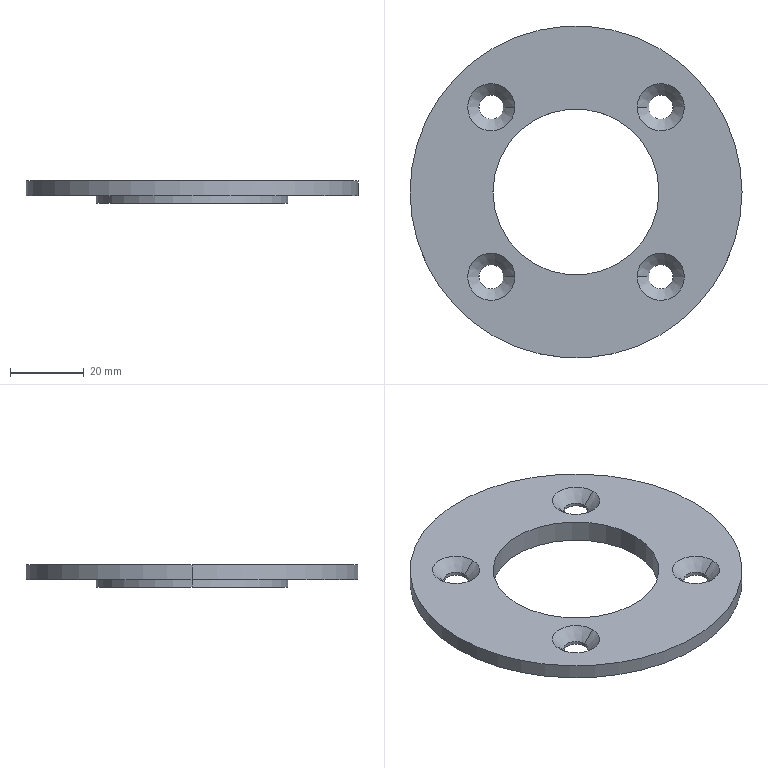Part | SolidWorks | features BaseBody 1 | 1 solid | 25 faces | box 90 x 90 x 6 mm | volume 19081 mm3 | cylinder 14 | cone 8 | plane 3 | commonest cylinder face diameters 6.6 x8 45 x2 52 x2 90 x2
STEP:
#1=CARTESIAN_POINT('',(200.547,1592.079,-382.));
#2=VERTEX_POINT('',#1);
#3=CARTESIAN_POINT('',(155.547,1592.079,-382.));
#4=VERTEX_POINT('',#3);
#5=CARTESIAN_POINT('',(178.047,1592.079,-382.));
#6=DIRECTION('',(0.,0.,-1.));
#7=DIRECTION('',(-1.,0.,0.));
#8=AXIS2_PLACEMENT_3D('',#5,#6,#7);
#9=CIRCLE('',#8,22.5);
#10=EDGE_CURVE('',#2,#4,#9,.T.);
#11=ORIENTED_EDGE('',*,*,#10,.F.);
#12=CARTESIAN_POINT('',(200.547,1592.079,-388.));
#13=VERTEX_POINT('',#12);
#14=CARTESIAN_POINT('',(200.547,1592.079,-382.));
#15=DIRECTION('',(0.,0.,-1.));
#16=VECTOR('',#15,1000.);
#17=LINE('',#14,#16);
#18=EDGE_CURVE('',#2,#13,#17,.T.);
#19=ORIENTED_EDGE('',*,*,#18,.T.);
#20=CARTESIAN_POINT('',(155.547,1592.079,-388.));
#21=VERTEX_POINT('',#20);
#22=CARTESIAN_POINT('',(178.047,1592.079,-388.));
#23=DIRECTION('',(0.,0.,1.));
#24=DIRECTION('',(-1.,0.,0.));
#25=AXIS2_PLACEMENT_3D('',#22,#23,#24);
#26=CIRCLE('',#25,22.5);
#27=EDGE_CURVE('',#21,#13,#26,.T.);
#28=ORIENTED_EDGE('',*,*,#27,.F.);
#29=CARTESIAN_POINT('',(155.547,1592.079,-382.));
#30=DIRECTION('',(0.,0.,-1.));
#31=VECTOR('',#30,1000.);
#32=LINE('',#29,#31);
#33=EDGE_CURVE('',#4,#21,#32,.T.);
#34=ORIENTED_EDGE('',*,*,#33,.F.);
#35=EDGE_LOOP('',(#11,#19,#28,#34));
#36=FACE_OUTER_BOUND('',#35,.T.);
#37=CARTESIAN_POINT('',(178.047,1592.079,-382.));
#38=DIRECTION('',(0.,0.,-1.));
#39=DIRECTION('',(-1.,0.,0.));
#40=AXIS2_PLACEMENT_3D('',#37,#38,#39);
#41=CYLINDRICAL_SURFACE('',#40,22.5);
#42=ADVANCED_FACE('',(#36),#41,.F.);
#43=CARTESIAN_POINT('',(151.766,1615.06,-385.1));
#44=VERTEX_POINT('',#43);
#45=CARTESIAN_POINT('',(158.366,1615.06,-385.1));
#46=VERTEX_POINT('',#45);
#47=CARTESIAN_POINT('',(155.066,1615.06,-385.1));
#48=DIRECTION('',(0.,0.,1.));
#49=DIRECTION('',(-0.7071,0.7071,0.));
#50=AXIS2_PLACEMENT_3D('',#47,#48,#49);
#51=CIRCLE('',#50,3.3);
#52=EDGE_CURVE('',#44,#46,#51,.T.);
#53=ORIENTED_EDGE('',*,*,#52,.F.);
#54=CARTESIAN_POINT('',(148.666,1615.06,-382.));
#55=VERTEX_POINT('',#54);
#56=CARTESIAN_POINT('',(148.666,1615.06,-382.));
#57=DIRECTION('',(-0.7071,0.,0.7071));
#58=VECTOR('',#57,1000.);
#59=LINE('',#56,#58);
#60=EDGE_CURVE('',#44,#55,#59,.T.);
#61=ORIENTED_EDGE('',*,*,#60,.T.);
#62=CARTESIAN_POINT('',(161.466,1615.06,-382.));
#63=VERTEX_POINT('',#62);
#64=CARTESIAN_POINT('',(155.066,1615.06,-382.));
#65=DIRECTION('',(0.,0.,-1.));
#66=DIRECTION('',(1.,0.,0.));
#67=AXIS2_PLACEMENT_3D('',#64,#65,#66);
#68=CIRCLE('',#67,6.4);
#69=EDGE_CURVE('',#63,#55,#68,.T.);
#70=ORIENTED_EDGE('',*,*,#69,.F.);
#71=CARTESIAN_POINT('',(161.466,1615.06,-382.));
#72=DIRECTION('',(0.7071,0.,0.7071));
#73=VECTOR('',#72,1000.);
#74=LINE('',#71,#73);
#75=EDGE_CURVE('',#46,#63,#74,.T.);
#76=ORIENTED_EDGE('',*,*,#75,.F.);
#77=EDGE_LOOP('',(#53,#61,#70,#76));
#78=FACE_OUTER_BOUND('',#77,.T.);
#79=CARTESIAN_POINT('',(155.066,1615.06,-382.));
#80=DIRECTION('',(0.,0.,1.));
#81=DIRECTION('',(1.,0.,0.));
#82=AXIS2_PLACEMENT_3D('',#79,#80,#81);
#83=CONICAL_SURFACE('',#82,6.4,0.7854);
#84=ADVANCED_FACE('',(#78),#83,.F.);
#85=CARTESIAN_POINT('',(197.727,1615.06,-385.1));
#86=VERTEX_POINT('',#85);
#87=CARTESIAN_POINT('',(204.327,1615.06,-385.1));
#88=VERTEX_POINT('',#87);
#89=CARTESIAN_POINT('',(201.027,1615.06,-385.1));
#90=DIRECTION('',(0.,0.,1.));
#91=DIRECTION('',(-0.7071,0.7071,0.));
#92=AXIS2_PLACEMENT_3D('',#89,#90,#91);
#93=CIRCLE('',#92,3.3);
#94=EDGE_CURVE('',#86,#88,#93,.T.);
#95=ORIENTED_EDGE('',*,*,#94,.F.);
#96=CARTESIAN_POINT('',(194.627,1615.06,-382.));
#97=VERTEX_POINT('',#96);
#98=CARTESIAN_POINT('',(194.627,1615.06,-382.));
#99=DIRECTION('',(-0.7071,0.,0.7071));
#100=VECTOR('',#99,1000.);
#101=LINE('',#98,#100);
#102=EDGE_CURVE('',#86,#97,#101,.T.);
#103=ORIENTED_EDGE('',*,*,#102,.T.);
#104=CARTESIAN_POINT('',(207.427,1615.06,-382.));
#105=VERTEX_POINT('',#104);
#106=CARTESIAN_POINT('',(201.027,1615.06,-382.));
#107=DIRECTION('',(0.,0.,-1.));
#108=DIRECTION('',(1.,0.,0.));
#109=AXIS2_PLACEMENT_3D('',#106,#107,#108);
#110=CIRCLE('',#109,6.4);
#111=EDGE_CURVE('',#105,#97,#110,.T.);
#112=ORIENTED_EDGE('',*,*,#111,.F.);
#113=CARTESIAN_POINT('',(207.427,1615.06,-382.));
#114=DIRECTION('',(0.7071,0.,0.7071));
#115=VECTOR('',#114,1000.);
#116=LINE('',#113,#115);
#117=EDGE_CURVE('',#88,#105,#116,.T.);
#118=ORIENTED_EDGE('',*,*,#117,.F.);
#119=EDGE_LOOP('',(#95,#103,#112,#118));
#120=FACE_OUTER_BOUND('',#119,.T.);
#121=CARTESIAN_POINT('',(201.027,1615.06,-382.));
#122=DIRECTION('',(0.,0.,1.));
#123=DIRECTION('',(1.,0.,0.));
#124=AXIS2_PLACEMENT_3D('',#121,#122,#123);
#125=CONICAL_SURFACE('',#124,6.4,0.7854);
#126=ADVANCED_FACE('',(#120),#125,.F.);
#127=CARTESIAN_POINT('',(197.727,1569.098,-385.1));
#128=VERTEX_POINT('',#127);
#129=CARTESIAN_POINT('',(204.327,1569.098,-385.1));
#130=VERTEX_POINT('',#129);
#131=CARTESIAN_POINT('',(201.027,1569.098,-385.1));
#132=DIRECTION('',(0.,0.,1.));
#133=DIRECTION('',(-0.7071,0.7071,0.));
#134=AXIS2_PLACEMENT_3D('',#131,#132,#133);
#135=CIRCLE('',#134,3.3);
#136=EDGE_CURVE('',#128,#130,#135,.T.);
#137=ORIENTED_EDGE('',*,*,#136,.F.);
#138=CARTESIAN_POINT('',(194.627,1569.098,-382.));
#139=VERTEX_POINT('',#138);
#140=CARTESIAN_POINT('',(194.627,1569.098,-382.));
#141=DIRECTION('',(-0.7071,0.,0.7071));
#142=VECTOR('',#141,1000.);
#143=LINE('',#140,#142);
#144=EDGE_CURVE('',#128,#139,#143,.T.);
#145=ORIENTED_EDGE('',*,*,#144,.T.);
#146=CARTESIAN_POINT('',(207.427,1569.098,-382.));
#147=VERTEX_POINT('',#146);
#148=CARTESIAN_POINT('',(201.027,1569.098,-382.));
#149=DIRECTION('',(0.,0.,-1.));
#150=DIRECTION('',(1.,0.,0.));
#151=AXIS2_PLACEMENT_3D('',#148,#149,#150);
#152=CIRCLE('',#151,6.4);
#153=EDGE_CURVE('',#147,#139,#152,.T.);
#154=ORIENTED_EDGE('',*,*,#153,.F.);
#155=CARTESIAN_POINT('',(207.427,1569.098,-382.));
#156=DIRECTION('',(0.7071,0.,0.7071));
#157=VECTOR('',#156,1000.);
#158=LINE('',#155,#157);
#159=EDGE_CURVE('',#130,#147,#158,.T.);
#160=ORIENTED_EDGE('',*,*,#159,.F.);
#161=EDGE_LOOP('',(#137,#145,#154,#160));
#162=FACE_OUTER_BOUND('',#161,.T.);
#163=CARTESIAN_POINT('',(201.027,1569.098,-382.));
#164=DIRECTION('',(0.,0.,1.));
#165=DIRECTION('',(1.,0.,0.));
#166=AXIS2_PLACEMENT_3D('',#163,#164,#165);
#167=CONICAL_SURFACE('',#166,6.4,0.7854);
#168=ADVANCED_FACE('',(#162),#167,.F.);
#169=CARTESIAN_POINT('',(151.766,1569.098,-385.1));
#170=VERTEX_POINT('',#169);
#171=CARTESIAN_POINT('',(158.366,1569.098,-385.1));
#172=VERTEX_POINT('',#171);
#173=CARTESIAN_POINT('',(155.066,1569.098,-385.1));
#174=DIRECTION('',(0.,0.,1.));
#175=DIRECTION('',(-0.7071,0.7071,0.));
#176=AXIS2_PLACEMENT_3D('',#173,#174,#175);
#177=CIRCLE('',#176,3.3);
#178=EDGE_CURVE('',#170,#172,#177,.T.);
#179=ORIENTED_EDGE('',*,*,#178,.F.);
#180=CARTESIAN_POINT('',(148.666,1569.098,-382.));
#181=VERTEX_POINT('',#180);
#182=CARTESIAN_POINT('',(148.666,1569.098,-382.));
#183=DIRECTION('',(-0.7071,0.,0.7071));
#184=VECTOR('',#183,1000.);
#185=LINE('',#182,#184);
#186=EDGE_CURVE('',#170,#181,#185,.T.);
#187=ORIENTED_EDGE('',*,*,#186,.T.);
#188=CARTESIAN_POINT('',(161.466,1569.098,-382.));
#189=VERTEX_POINT('',#188);
#190=CARTESIAN_POINT('',(155.066,1569.098,-382.));
#191=DIRECTION('',(0.,0.,-1.));
#192=DIRECTION('',(1.,0.,0.));
#193=AXIS2_PLACEMENT_3D('',#190,#191,#192);
#194=CIRCLE('',#193,6.4);
#195=EDGE_CURVE('',#189,#181,#194,.T.);
#196=ORIENTED_EDGE('',*,*,#195,.F.);
#197=CARTESIAN_POINT('',(161.466,1569.098,-382.));
#198=DIRECTION('',(0.7071,0.,0.7071));
#199=VECTOR('',#198,1000.);
#200=LINE('',#197,#199);
#201=EDGE_CURVE('',#172,#189,#200,.T.);
#202=ORIENTED_EDGE('',*,*,#201,.F.);
#203=EDGE_LOOP('',(#179,#187,#196,#202));
#204=FACE_OUTER_BOUND('',#203,.T.);
#205=CARTESIAN_POINT('',(155.066,1569.098,-382.));
#206=DIRECTION('',(0.,0.,1.));
#207=DIRECTION('',(1.,0.,0.));
#208=AXIS2_PLACEMENT_3D('',#205,#206,#207);
#209=CONICAL_SURFACE('',#208,6.4,0.7854);
#210=ADVANCED_FACE('',(#204),#209,.F.);
#211=CARTESIAN_POINT('',(223.047,1592.079,-382.));
#212=VERTEX_POINT('',#211);
#213=CARTESIAN_POINT('',(133.047,1592.079,-382.));
#214=VERTEX_POINT('',#213);
#215=CARTESIAN_POINT('',(178.047,1592.079,-382.));
#216=DIRECTION('',(0.,0.,1.));
#217=DIRECTION('',(-1.,0.,0.));
#218=AXIS2_PLACEMENT_3D('',#215,#216,#217);
#219=CIRCLE('',#218,45.);
#220=EDGE_CURVE('',#212,#214,#219,.T.);
#221=ORIENTED_EDGE('',*,*,#220,.F.);
#222=CARTESIAN_POINT('',(223.047,1592.079,-386.));
#223=VERTEX_POINT('',#222);
#224=CARTESIAN_POINT('',(223.047,1592.079,-382.));
#225=DIRECTION('',(0.,0.,-1.));
#226=VECTOR('',#225,1000.);
#227=LINE('',#224,#226);
#228=EDGE_CURVE('',#212,#223,#227,.T.);
#229=ORIENTED_EDGE('',*,*,#228,.T.);
#230=CARTESIAN_POINT('',(133.047,1592.079,-386.));
#231=VERTEX_POINT('',#230);
#232=CARTESIAN_POINT('',(178.047,1592.079,-386.));
#233=DIRECTION('',(0.,0.,1.));
#234=DIRECTION('',(-1.,0.,0.));
#235=AXIS2_PLACEMENT_3D('',#232,#233,#234);
#236=CIRCLE('',#235,45.);
#237=EDGE_CURVE('',#223,#231,#236,.T.);
#238=ORIENTED_EDGE('',*,*,#237,.T.);
#239=CARTESIAN_POINT('',(133.047,1592.079,-382.));
#240=DIRECTION('',(0.,0.,-1.));
#241=VECTOR('',#240,1000.);
#242=LINE('',#239,#241);
#243=EDGE_CURVE('',#214,#231,#242,.T.);
#244=ORIENTED_EDGE('',*,*,#243,.F.);
#245=EDGE_LOOP('',(#221,#229,#238,#244));
#246=FACE_OUTER_BOUND('',#245,.T.);
#247=CARTESIAN_POINT('',(178.047,1592.079,-382.));
#248=DIRECTION('',(0.,0.,-1.));
#249=DIRECTION('',(-1.,0.,0.));
#250=AXIS2_PLACEMENT_3D('',#247,#248,#249);
#251=CYLINDRICAL_SURFACE('',#250,45.);
#252=ADVANCED_FACE('',(#246),#251,.T.);
#253=CARTESIAN_POINT('',(151.766,1615.06,-386.));
#254=VERTEX_POINT('',#253);
#255=CARTESIAN_POINT('',(158.366,1615.06,-386.));
#256=VERTEX_POINT('',#255);
#257=CARTESIAN_POINT('',(155.066,1615.06,-386.));
#258=DIRECTION('',(0.,0.,1.));
#259=DIRECTION('',(1.,0.,0.));
#260=AXIS2_PLACEMENT_3D('',#257,#258,#259);
#261=CIRCLE('',#260,3.3);
#262=EDGE_CURVE('',#254,#256,#261,.T.);
#263=ORIENTED_EDGE('',*,*,#262,.F.);
#264=CARTESIAN_POINT('',(151.766,1615.06,-382.));
#265=DIRECTION('',(0.,0.,1.));
#266=VECTOR('',#265,1000.);
#267=LINE('',#264,#266);
#268=EDGE_CURVE('',#254,#44,#267,.T.);
#269=ORIENTED_EDGE('',*,*,#268,.T.);
#270=ORIENTED_EDGE('',*,*,#52,.T.);
#271=CARTESIAN_POINT('',(158.366,1615.06,-382.));
#272=DIRECTION('',(0.,0.,1.));
#273=VECTOR('',#272,1000.);
#274=LINE('',#271,#273);
#275=EDGE_CURVE('',#256,#46,#274,.T.);
#276=ORIENTED_EDGE('',*,*,#275,.F.);
#277=EDGE_LOOP('',(#263,#269,#270,#276));
#278=FACE_OUTER_BOUND('',#277,.T.);
#279=CARTESIAN_POINT('',(155.066,1615.06,-382.));
#280=DIRECTION('',(0.,0.,1.));
#281=DIRECTION('',(1.,0.,0.));
#282=AXIS2_PLACEMENT_3D('',#279,#280,#281);
#283=CYLINDRICAL_SURFACE('',#282,3.3);
#284=ADVANCED_FACE('',(#278),#283,.F.);
#285=CARTESIAN_POINT('',(197.727,1615.06,-386.));
#286=VERTEX_POINT('',#285);
#287=CARTESIAN_POINT('',(204.327,1615.06,-386.));
#288=VERTEX_POINT('',#287);
#289=CARTESIAN_POINT('',(201.027,1615.06,-386.));
#290=DIRECTION('',(0.,0.,1.));
#291=DIRECTION('',(1.,0.,0.));
#292=AXIS2_PLACEMENT_3D('',#289,#290,#291);
#293=CIRCLE('',#292,3.3);
#294=EDGE_CURVE('',#286,#288,#293,.T.);
#295=ORIENTED_EDGE('',*,*,#294,.F.);
#296=CARTESIAN_POINT('',(197.727,1615.06,-382.));
#297=DIRECTION('',(0.,0.,1.));
#298=VECTOR('',#297,1000.);
#299=LINE('',#296,#298);
#300=EDGE_CURVE('',#286,#86,#299,.T.);
#301=ORIENTED_EDGE('',*,*,#300,.T.);
#302=ORIENTED_EDGE('',*,*,#94,.T.);
#303=CARTESIAN_POINT('',(204.327,1615.06,-382.));
#304=DIRECTION('',(0.,0.,1.));
#305=VECTOR('',#304,1000.);
#306=LINE('',#303,#305);
#307=EDGE_CURVE('',#288,#88,#306,.T.);
#308=ORIENTED_EDGE('',*,*,#307,.F.);
#309=EDGE_LOOP('',(#295,#301,#302,#308));
#310=FACE_OUTER_BOUND('',#309,.T.);
#311=CARTESIAN_POINT('',(201.027,1615.06,-382.));
#312=DIRECTION('',(0.,0.,1.));
#313=DIRECTION('',(1.,0.,0.));
#314=AXIS2_PLACEMENT_3D('',#311,#312,#313);
#315=CYLINDRICAL_SURFACE('',#314,3.3);
#316=ADVANCED_FACE('',(#310),#315,.F.);
#317=CARTESIAN_POINT('',(197.727,1569.098,-386.));
#318=VERTEX_POINT('',#317);
#319=CARTESIAN_POINT('',(204.327,1569.098,-386.));
#320=VERTEX_POINT('',#319);
#321=CARTESIAN_POINT('',(201.027,1569.098,-386.));
#322=DIRECTION('',(0.,0.,1.));
#323=DIRECTION('',(1.,0.,0.));
#324=AXIS2_PLACEMENT_3D('',#321,#322,#323);
#325=CIRCLE('',#324,3.3);
#326=EDGE_CURVE('',#318,#320,#325,.T.);
#327=ORIENTED_EDGE('',*,*,#326,.F.);
#328=CARTESIAN_POINT('',(197.727,1569.098,-382.));
#329=DIRECTION('',(0.,0.,1.));
#330=VECTOR('',#329,1000.);
#331=LINE('',#328,#330);
#332=EDGE_CURVE('',#318,#128,#331,.T.);
#333=ORIENTED_EDGE('',*,*,#332,.T.);
#334=ORIENTED_EDGE('',*,*,#136,.T.);
#335=CARTESIAN_POINT('',(204.327,1569.098,-382.));
#336=DIRECTION('',(0.,0.,1.));
#337=VECTOR('',#336,1000.);
#338=LINE('',#335,#337);
#339=EDGE_CURVE('',#320,#130,#338,.T.);
#340=ORIENTED_EDGE('',*,*,#339,.F.);
#341=EDGE_LOOP('',(#327,#333,#334,#340));
#342=FACE_OUTER_BOUND('',#341,.T.);
#343=CARTESIAN_POINT('',(201.027,1569.098,-382.));
#344=DIRECTION('',(0.,0.,1.));
#345=DIRECTION('',(1.,0.,0.));
#346=AXIS2_PLACEMENT_3D('',#343,#344,#345);
#347=CYLINDRICAL_SURFACE('',#346,3.3);
#348=ADVANCED_FACE('',(#342),#347,.F.);
#349=CARTESIAN_POINT('',(151.766,1569.098,-386.));
#350=VERTEX_POINT('',#349);
#351=CARTESIAN_POINT('',(158.366,1569.098,-386.));
#352=VERTEX_POINT('',#351);
#353=CARTESIAN_POINT('',(155.066,1569.098,-386.));
#354=DIRECTION('',(0.,0.,1.));
#355=DIRECTION('',(1.,0.,0.));
#356=AXIS2_PLACEMENT_3D('',#353,#354,#355);
#357=CIRCLE('',#356,3.3);
#358=EDGE_CURVE('',#350,#352,#357,.T.);
#359=ORIENTED_EDGE('',*,*,#358,.F.);
#360=CARTESIAN_POINT('',(151.766,1569.098,-382.));
#361=DIRECTION('',(0.,0.,1.));
#362=VECTOR('',#361,1000.);
#363=LINE('',#360,#362);
#364=EDGE_CURVE('',#350,#170,#363,.T.);
#365=ORIENTED_EDGE('',*,*,#364,.T.);
#366=ORIENTED_EDGE('',*,*,#178,.T.);
#367=CARTESIAN_POINT('',(158.366,1569.098,-382.));
#368=DIRECTION('',(0.,0.,1.));
#369=VECTOR('',#368,1000.);
#370=LINE('',#367,#369);
#371=EDGE_CURVE('',#352,#172,#370,.T.);
#372=ORIENTED_EDGE('',*,*,#371,.F.);
#373=EDGE_LOOP('',(#359,#365,#366,#372));
#374=FACE_OUTER_BOUND('',#373,.T.);
#375=CARTESIAN_POINT('',(155.066,1569.098,-382.));
#376=DIRECTION('',(0.,0.,1.));
#377=DIRECTION('',(1.,0.,0.));
#378=AXIS2_PLACEMENT_3D('',#375,#376,#377);
#379=CYLINDRICAL_SURFACE('',#378,3.3);
#380=ADVANCED_FACE('',(#374),#379,.F.);
#381=CARTESIAN_POINT('',(204.047,1592.079,-386.));
#382=VERTEX_POINT('',#381);
#383=CARTESIAN_POINT('',(152.047,1592.079,-386.));
#384=VERTEX_POINT('',#383);
#385=CARTESIAN_POINT('',(178.047,1592.079,-386.));
#386=DIRECTION('',(0.,0.,1.));
#387=DIRECTION('',(-1.,0.,0.));
#388=AXIS2_PLACEMENT_3D('',#385,#386,#387);
#389=CIRCLE('',#388,26.);
#390=EDGE_CURVE('',#382,#384,#389,.T.);
#391=ORIENTED_EDGE('',*,*,#390,.F.);
#392=CARTESIAN_POINT('',(204.047,1592.079,-388.));
#393=VERTEX_POINT('',#392);
#394=CARTESIAN_POINT('',(204.047,1592.079,-386.));
#395=DIRECTION('',(0.,0.,-1.));
#396=VECTOR('',#395,1000.);
#397=LINE('',#394,#396);
#398=EDGE_CURVE('',#382,#393,#397,.T.);
#399=ORIENTED_EDGE('',*,*,#398,.T.);
#400=CARTESIAN_POINT('',(152.047,1592.079,-388.));
#401=VERTEX_POINT('',#400);
#402=CARTESIAN_POINT('',(178.047,1592.079,-388.));
#403=DIRECTION('',(0.,0.,1.));
#404=DIRECTION('',(-1.,0.,0.));
#405=AXIS2_PLACEMENT_3D('',#402,#403,#404);
#406=CIRCLE('',#405,26.);
#407=EDGE_CURVE('',#393,#401,#406,.T.);
#408=ORIENTED_EDGE('',*,*,#407,.T.);
#409=CARTESIAN_POINT('',(152.047,1592.079,-386.));
#410=DIRECTION('',(0.,0.,-1.));
#411=VECTOR('',#410,1000.);
#412=LINE('',#409,#411);
#413=EDGE_CURVE('',#384,#401,#412,.T.);
#414=ORIENTED_EDGE('',*,*,#413,.F.);
#415=EDGE_LOOP('',(#391,#399,#408,#414));
#416=FACE_OUTER_BOUND('',#415,.T.);
#417=CARTESIAN_POINT('',(178.047,1592.079,-386.));
#418=DIRECTION('',(0.,0.,-1.));
#419=DIRECTION('',(-1.,0.,0.));
#420=AXIS2_PLACEMENT_3D('',#417,#418,#419);
#421=CYLINDRICAL_SURFACE('',#420,26.);
#422=ADVANCED_FACE('',(#416),#421,.T.);
#423=CARTESIAN_POINT('',(178.047,1592.079,-382.));
#424=DIRECTION('',(0.,0.,-1.));
#425=DIRECTION('',(-1.,0.,0.));
#426=AXIS2_PLACEMENT_3D('',#423,#424,#425);
#427=CIRCLE('',#426,22.5);
#428=EDGE_CURVE('',#4,#2,#427,.T.);
#429=ORIENTED_EDGE('',*,*,#428,.T.);
#430=ORIENTED_EDGE('',*,*,#10,.T.);
#431=EDGE_LOOP('',(#429,#430));
#432=FACE_BOUND('',#431,.T.);
#433=ORIENTED_EDGE('',*,*,#69,.T.);
#434=CARTESIAN_POINT('',(155.066,1615.06,-382.));
#435=DIRECTION('',(0.,0.,-1.));
#436=DIRECTION('',(1.,0.,0.));
#437=AXIS2_PLACEMENT_3D('',#434,#435,#436);
#438=CIRCLE('',#437,6.4);
#439=EDGE_CURVE('',#55,#63,#438,.T.);
#440=ORIENTED_EDGE('',*,*,#439,.T.);
#441=EDGE_LOOP('',(#433,#440));
#442=FACE_BOUND('',#441,.T.);
#443=ORIENTED_EDGE('',*,*,#111,.T.);
#444=CARTESIAN_POINT('',(201.027,1615.06,-382.));
#445=DIRECTION('',(0.,0.,-1.));
#446=DIRECTION('',(1.,0.,0.));
#447=AXIS2_PLACEMENT_3D('',#444,#445,#446);
#448=CIRCLE('',#447,6.4);
#449=EDGE_CURVE('',#97,#105,#448,.T.);
#450=ORIENTED_EDGE('',*,*,#449,.T.);
#451=EDGE_LOOP('',(#443,#450));
#452=FACE_BOUND('',#451,.T.);
#453=ORIENTED_EDGE('',*,*,#153,.T.);
#454=CARTESIAN_POINT('',(201.027,1569.098,-382.));
#455=DIRECTION('',(0.,0.,-1.));
#456=DIRECTION('',(1.,0.,0.));
#457=AXIS2_PLACEMENT_3D('',#454,#455,#456);
#458=CIRCLE('',#457,6.4);
#459=EDGE_CURVE('',#139,#147,#458,.T.);
#460=ORIENTED_EDGE('',*,*,#459,.T.);
#461=EDGE_LOOP('',(#453,#460));
#462=FACE_BOUND('',#461,.T.);
#463=ORIENTED_EDGE('',*,*,#195,.T.);
#464=CARTESIAN_POINT('',(155.066,1569.098,-382.));
#465=DIRECTION('',(0.,0.,-1.));
#466=DIRECTION('',(1.,0.,0.));
#467=AXIS2_PLACEMENT_3D('',#464,#465,#466);
#468=CIRCLE('',#467,6.4);
#469=EDGE_CURVE('',#181,#189,#468,.T.);
#470=ORIENTED_EDGE('',*,*,#469,.T.);
#471=EDGE_LOOP('',(#463,#470));
#472=FACE_BOUND('',#471,.T.);
#473=CARTESIAN_POINT('',(178.047,1592.079,-382.));
#474=DIRECTION('',(0.,0.,1.));
#475=DIRECTION('',(-1.,0.,0.));
#476=AXIS2_PLACEMENT_3D('',#473,#474,#475);
#477=CIRCLE('',#476,45.);
#478=EDGE_CURVE('',#214,#212,#477,.T.);
#479=ORIENTED_EDGE('',*,*,#478,.T.);
#480=ORIENTED_EDGE('',*,*,#220,.T.);
#481=EDGE_LOOP('',(#479,#480));
#482=FACE_OUTER_BOUND('',#481,.T.);
#483=CARTESIAN_POINT('',(178.047,1592.079,-382.));
#484=DIRECTION('',(0.,0.,1.));
#485=DIRECTION('',(1.,0.,0.));
#486=AXIS2_PLACEMENT_3D('',#483,#484,#485);
#487=PLANE('',#486);
#488=ADVANCED_FACE('',(#432,#442,#452,#462,#472,#482),#487,.T.);
#489=ORIENTED_EDGE('',*,*,#18,.F.);
#490=ORIENTED_EDGE('',*,*,#428,.F.);
#491=ORIENTED_EDGE('',*,*,#33,.T.);
#492=CARTESIAN_POINT('',(178.047,1592.079,-388.));
#493=DIRECTION('',(0.,0.,1.));
#494=DIRECTION('',(-1.,0.,0.));
#495=AXIS2_PLACEMENT_3D('',#492,#493,#494);
#496=CIRCLE('',#495,22.5);
#497=EDGE_CURVE('',#13,#21,#496,.T.);
#498=ORIENTED_EDGE('',*,*,#497,.F.);
#499=EDGE_LOOP('',(#489,#490,#491,#498));
#500=FACE_OUTER_BOUND('',#499,.T.);
#501=CARTESIAN_POINT('',(178.047,1592.079,-382.));
#502=DIRECTION('',(0.,0.,-1.));
#503=DIRECTION('',(-1.,0.,0.));
#504=AXIS2_PLACEMENT_3D('',#501,#502,#503);
#505=CYLINDRICAL_SURFACE('',#504,22.5);
#506=ADVANCED_FACE('',(#500),#505,.F.);
#507=ORIENTED_EDGE('',*,*,#60,.F.);
#508=CARTESIAN_POINT('',(155.066,1615.06,-385.1));
#509=DIRECTION('',(0.,0.,1.));
#510=DIRECTION('',(-0.7071,0.7071,0.));
#511=AXIS2_PLACEMENT_3D('',#508,#509,#510);
#512=CIRCLE('',#511,3.3);
#513=EDGE_CURVE('',#46,#44,#512,.T.);
#514=ORIENTED_EDGE('',*,*,#513,.F.);
#515=ORIENTED_EDGE('',*,*,#75,.T.);
#516=ORIENTED_EDGE('',*,*,#439,.F.);
#517=EDGE_LOOP('',(#507,#514,#515,#516));
#518=FACE_OUTER_BOUND('',#517,.T.);
#519=CARTESIAN_POINT('',(155.066,1615.06,-382.));
#520=DIRECTION('',(0.,0.,1.));
#521=DIRECTION('',(1.,0.,0.));
#522=AXIS2_PLACEMENT_3D('',#519,#520,#521);
#523=CONICAL_SURFACE('',#522,6.4,0.7854);
#524=ADVANCED_FACE('',(#518),#523,.F.);
#525=ORIENTED_EDGE('',*,*,#102,.F.);
#526=CARTESIAN_POINT('',(201.027,1615.06,-385.1));
#527=DIRECTION('',(0.,0.,1.));
#528=DIRECTION('',(-0.7071,0.7071,0.));
#529=AXIS2_PLACEMENT_3D('',#526,#527,#528);
#530=CIRCLE('',#529,3.3);
#531=EDGE_CURVE('',#88,#86,#530,.T.);
#532=ORIENTED_EDGE('',*,*,#531,.F.);
#533=ORIENTED_EDGE('',*,*,#117,.T.);
#534=ORIENTED_EDGE('',*,*,#449,.F.);
#535=EDGE_LOOP('',(#525,#532,#533,#534));
#536=FACE_OUTER_BOUND('',#535,.T.);
#537=CARTESIAN_POINT('',(201.027,1615.06,-382.));
#538=DIRECTION('',(0.,0.,1.));
#539=DIRECTION('',(1.,0.,0.));
#540=AXIS2_PLACEMENT_3D('',#537,#538,#539);
#541=CONICAL_SURFACE('',#540,6.4,0.7854);
#542=ADVANCED_FACE('',(#536),#541,.F.);
#543=ORIENTED_EDGE('',*,*,#144,.F.);
#544=CARTESIAN_POINT('',(201.027,1569.098,-385.1));
#545=DIRECTION('',(0.,0.,1.));
#546=DIRECTION('',(-0.7071,0.7071,0.));
#547=AXIS2_PLACEMENT_3D('',#544,#545,#546);
#548=CIRCLE('',#547,3.3);
#549=EDGE_CURVE('',#130,#128,#548,.T.);
#550=ORIENTED_EDGE('',*,*,#549,.F.);
#551=ORIENTED_EDGE('',*,*,#159,.T.);
#552=ORIENTED_EDGE('',*,*,#459,.F.);
#553=EDGE_LOOP('',(#543,#550,#551,#552));
#554=FACE_OUTER_BOUND('',#553,.T.);
#555=CARTESIAN_POINT('',(201.027,1569.098,-382.));
#556=DIRECTION('',(0.,0.,1.));
#557=DIRECTION('',(1.,0.,0.));
#558=AXIS2_PLACEMENT_3D('',#555,#556,#557);
#559=CONICAL_SURFACE('',#558,6.4,0.7854);
#560=ADVANCED_FACE('',(#554),#559,.F.);
#561=ORIENTED_EDGE('',*,*,#186,.F.);
#562=CARTESIAN_POINT('',(155.066,1569.098,-385.1));
#563=DIRECTION('',(0.,0.,1.));
#564=DIRECTION('',(-0.7071,0.7071,0.));
#565=AXIS2_PLACEMENT_3D('',#562,#563,#564);
#566=CIRCLE('',#565,3.3);
#567=EDGE_CURVE('',#172,#170,#566,.T.);
#568=ORIENTED_EDGE('',*,*,#567,.F.);
#569=ORIENTED_EDGE('',*,*,#201,.T.);
#570=ORIENTED_EDGE('',*,*,#469,.F.);
#571=EDGE_LOOP('',(#561,#568,#569,#570));
#572=FACE_OUTER_BOUND('',#571,.T.);
#573=CARTESIAN_POINT('',(155.066,1569.098,-382.));
#574=DIRECTION('',(0.,0.,1.));
#575=DIRECTION('',(1.,0.,0.));
#576=AXIS2_PLACEMENT_3D('',#573,#574,#575);
#577=CONICAL_SURFACE('',#576,6.4,0.7854);
#578=ADVANCED_FACE('',(#572),#577,.F.);
#579=ORIENTED_EDGE('',*,*,#228,.F.);
#580=ORIENTED_EDGE('',*,*,#478,.F.);
#581=ORIENTED_EDGE('',*,*,#243,.T.);
#582=CARTESIAN_POINT('',(178.047,1592.079,-386.));
#583=DIRECTION('',(0.,0.,1.));
#584=DIRECTION('',(-1.,0.,0.));
#585=AXIS2_PLACEMENT_3D('',#582,#583,#584);
#586=CIRCLE('',#585,45.);
#587=EDGE_CURVE('',#231,#223,#586,.T.);
#588=ORIENTED_EDGE('',*,*,#587,.T.);
#589=EDGE_LOOP('',(#579,#580,#581,#588));
#590=FACE_OUTER_BOUND('',#589,.T.);
#591=CARTESIAN_POINT('',(178.047,1592.079,-382.));
#592=DIRECTION('',(0.,0.,-1.));
#593=DIRECTION('',(-1.,0.,0.));
#594=AXIS2_PLACEMENT_3D('',#591,#592,#593);
#595=CYLINDRICAL_SURFACE('',#594,45.);
#596=ADVANCED_FACE('',(#590),#595,.T.);
#597=ORIENTED_EDGE('',*,*,#27,.T.);
#598=ORIENTED_EDGE('',*,*,#497,.T.);
#599=EDGE_LOOP('',(#597,#598));
#600=FACE_BOUND('',#599,.T.);
#601=CARTESIAN_POINT('',(178.047,1592.079,-388.));
#602=DIRECTION('',(0.,0.,1.));
#603=DIRECTION('',(-1.,0.,0.));
#604=AXIS2_PLACEMENT_3D('',#601,#602,#603);
#605=CIRCLE('',#604,26.);
#606=EDGE_CURVE('',#401,#393,#605,.T.);
#607=ORIENTED_EDGE('',*,*,#606,.F.);
#608=ORIENTED_EDGE('',*,*,#407,.F.);
#609=EDGE_LOOP('',(#607,#608));
#610=FACE_OUTER_BOUND('',#609,.T.);
#611=CARTESIAN_POINT('',(178.047,1592.079,-388.));
#612=DIRECTION('',(0.,0.,1.));
#613=DIRECTION('',(1.,0.,0.));
#614=AXIS2_PLACEMENT_3D('',#611,#612,#613);
#615=PLANE('',#614);
#616=ADVANCED_FACE('',(#600,#610),#615,.F.);
#617=ORIENTED_EDGE('',*,*,#268,.F.);
#618=CARTESIAN_POINT('',(155.066,1615.06,-386.));
#619=DIRECTION('',(0.,0.,1.));
#620=DIRECTION('',(1.,0.,0.));
#621=AXIS2_PLACEMENT_3D('',#618,#619,#620);
#622=CIRCLE('',#621,3.3);
#623=EDGE_CURVE('',#256,#254,#622,.T.);
#624=ORIENTED_EDGE('',*,*,#623,.F.);
#625=ORIENTED_EDGE('',*,*,#275,.T.);
#626=ORIENTED_EDGE('',*,*,#513,.T.);
#627=EDGE_LOOP('',(#617,#624,#625,#626));
#628=FACE_OUTER_BOUND('',#627,.T.);
#629=CARTESIAN_POINT('',(155.066,1615.06,-382.));
#630=DIRECTION('',(0.,0.,1.));
#631=DIRECTION('',(1.,0.,0.));
#632=AXIS2_PLACEMENT_3D('',#629,#630,#631);
#633=CYLINDRICAL_SURFACE('',#632,3.3);
#634=ADVANCED_FACE('',(#628),#633,.F.);
#635=ORIENTED_EDGE('',*,*,#300,.F.);
#636=CARTESIAN_POINT('',(201.027,1615.06,-386.));
#637=DIRECTION('',(0.,0.,1.));
#638=DIRECTION('',(1.,0.,0.));
#639=AXIS2_PLACEMENT_3D('',#636,#637,#638);
#640=CIRCLE('',#639,3.3);
#641=EDGE_CURVE('',#288,#286,#640,.T.);
#642=ORIENTED_EDGE('',*,*,#641,.F.);
#643=ORIENTED_EDGE('',*,*,#307,.T.);
#644=ORIENTED_EDGE('',*,*,#531,.T.);
#645=EDGE_LOOP('',(#635,#642,#643,#644));
#646=FACE_OUTER_BOUND('',#645,.T.);
#647=CARTESIAN_POINT('',(201.027,1615.06,-382.));
#648=DIRECTION('',(0.,0.,1.));
#649=DIRECTION('',(1.,0.,0.));
#650=AXIS2_PLACEMENT_3D('',#647,#648,#649);
#651=CYLINDRICAL_SURFACE('',#650,3.3);
#652=ADVANCED_FACE('',(#646),#651,.F.);
#653=ORIENTED_EDGE('',*,*,#332,.F.);
#654=CARTESIAN_POINT('',(201.027,1569.098,-386.));
#655=DIRECTION('',(0.,0.,1.));
#656=DIRECTION('',(1.,0.,0.));
#657=AXIS2_PLACEMENT_3D('',#654,#655,#656);
#658=CIRCLE('',#657,3.3);
#659=EDGE_CURVE('',#320,#318,#658,.T.);
#660=ORIENTED_EDGE('',*,*,#659,.F.);
#661=ORIENTED_EDGE('',*,*,#339,.T.);
#662=ORIENTED_EDGE('',*,*,#549,.T.);
#663=EDGE_LOOP('',(#653,#660,#661,#662));
#664=FACE_OUTER_BOUND('',#663,.T.);
#665=CARTESIAN_POINT('',(201.027,1569.098,-382.));
#666=DIRECTION('',(0.,0.,1.));
#667=DIRECTION('',(1.,0.,0.));
#668=AXIS2_PLACEMENT_3D('',#665,#666,#667);
#669=CYLINDRICAL_SURFACE('',#668,3.3);
#670=ADVANCED_FACE('',(#664),#669,.F.);
#671=ORIENTED_EDGE('',*,*,#364,.F.);
#672=CARTESIAN_POINT('',(155.066,1569.098,-386.));
#673=DIRECTION('',(0.,0.,1.));
#674=DIRECTION('',(1.,0.,0.));
#675=AXIS2_PLACEMENT_3D('',#672,#673,#674);
#676=CIRCLE('',#675,3.3);
#677=EDGE_CURVE('',#352,#350,#676,.T.);
#678=ORIENTED_EDGE('',*,*,#677,.F.);
#679=ORIENTED_EDGE('',*,*,#371,.T.);
#680=ORIENTED_EDGE('',*,*,#567,.T.);
#681=EDGE_LOOP('',(#671,#678,#679,#680));
#682=FACE_OUTER_BOUND('',#681,.T.);
#683=CARTESIAN_POINT('',(155.066,1569.098,-382.));
#684=DIRECTION('',(0.,0.,1.));
#685=DIRECTION('',(1.,0.,0.));
#686=AXIS2_PLACEMENT_3D('',#683,#684,#685);
#687=CYLINDRICAL_SURFACE('',#686,3.3);
#688=ADVANCED_FACE('',(#682),#687,.F.);
#689=ORIENTED_EDGE('',*,*,#623,.T.);
#690=ORIENTED_EDGE('',*,*,#262,.T.);
#691=EDGE_LOOP('',(#689,#690));
#692=FACE_BOUND('',#691,.T.);
#693=CARTESIAN_POINT('',(178.047,1592.079,-386.));
#694=DIRECTION('',(0.,0.,1.));
#695=DIRECTION('',(-1.,0.,0.));
#696=AXIS2_PLACEMENT_3D('',#693,#694,#695);
#697=CIRCLE('',#696,26.);
#698=EDGE_CURVE('',#384,#382,#697,.T.);
#699=ORIENTED_EDGE('',*,*,#698,.T.);
#700=ORIENTED_EDGE('',*,*,#390,.T.);
#701=EDGE_LOOP('',(#699,#700));
#702=FACE_BOUND('',#701,.T.);
#703=ORIENTED_EDGE('',*,*,#641,.T.);
#704=ORIENTED_EDGE('',*,*,#294,.T.);
#705=EDGE_LOOP('',(#703,#704));
#706=FACE_BOUND('',#705,.T.);
#707=ORIENTED_EDGE('',*,*,#659,.T.);
#708=ORIENTED_EDGE('',*,*,#326,.T.);
#709=EDGE_LOOP('',(#707,#708));
#710=FACE_BOUND('',#709,.T.);
#711=ORIENTED_EDGE('',*,*,#677,.T.);
#712=ORIENTED_EDGE('',*,*,#358,.T.);
#713=EDGE_LOOP('',(#711,#712));
#714=FACE_BOUND('',#713,.T.);
#715=ORIENTED_EDGE('',*,*,#587,.F.);
#716=ORIENTED_EDGE('',*,*,#237,.F.);
#717=EDGE_LOOP('',(#715,#716));
#718=FACE_OUTER_BOUND('',#717,.T.);
#719=CARTESIAN_POINT('',(178.047,1592.079,-386.));
#720=DIRECTION('',(0.,0.,-1.));
#721=DIRECTION('',(-1.,0.,0.));
#722=AXIS2_PLACEMENT_3D('',#719,#720,#721);
#723=PLANE('',#722);
#724=ADVANCED_FACE('',(#692,#702,#706,#710,#714,#718),#723,.T.);
#725=ORIENTED_EDGE('',*,*,#398,.F.);
#726=ORIENTED_EDGE('',*,*,#698,.F.);
#727=ORIENTED_EDGE('',*,*,#413,.T.);
#728=ORIENTED_EDGE('',*,*,#606,.T.);
#729=EDGE_LOOP('',(#725,#726,#727,#728));
#730=FACE_OUTER_BOUND('',#729,.T.);
#731=CARTESIAN_POINT('',(178.047,1592.079,-386.));
#732=DIRECTION('',(0.,0.,-1.));
#733=DIRECTION('',(-1.,0.,0.));
#734=AXIS2_PLACEMENT_3D('',#731,#732,#733);
#735=CYLINDRICAL_SURFACE('',#734,26.);
#736=ADVANCED_FACE('',(#730),#735,.T.);
#737=CLOSED_SHELL('',(#42,#84,#126,#168,#210,#252,#284,#316,#348,#380,#422,#488,#506,#524,#542,#560,#578,#596,#616,#634,#652,#670,#688,#724,#736));
#738=MANIFOLD_SOLID_BREP('',#737);
#739=CARTESIAN_POINT('',(0.,0.,0.));
#740=DIRECTION('',(0.,0.,1.));
#741=DIRECTION('',(1.,0.,0.));
#742=AXIS2_PLACEMENT_3D('',#739,#740,#741);
#743=(LENGTH_UNIT()NAMED_UNIT(*)SI_UNIT(.MILLI.,.METRE.));
#744=UNCERTAINTY_MEASURE_WITH_UNIT(LENGTH_MEASURE(0.00001),#743,'','');
#745=(NAMED_UNIT(*)PLANE_ANGLE_UNIT()SI_UNIT($,.RADIAN.));
#746=(NAMED_UNIT(*)SI_UNIT($,.STERADIAN.)SOLID_ANGLE_UNIT());
#747=(GEOMETRIC_REPRESENTATION_CONTEXT(3)GLOBAL_UNCERTAINTY_ASSIGNED_CONTEXT((#744))GLOBAL_UNIT_ASSIGNED_CONTEXT((#743,#745,#746))REPRESENTATION_CONTEXT('',''));
#748=ADVANCED_BREP_SHAPE_REPRESENTATION('',(#738,#742),#747);